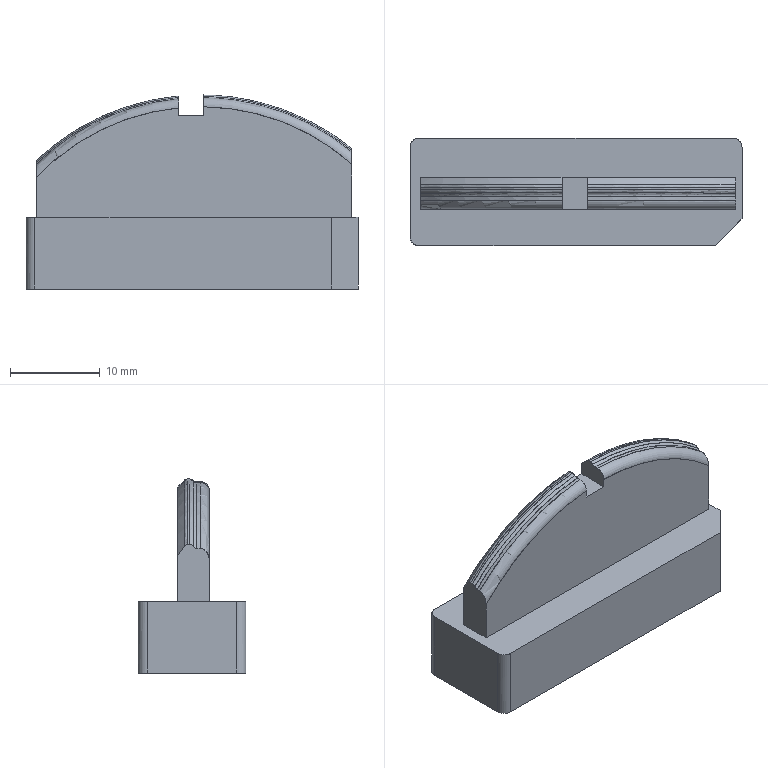NC program | PowerMill | posted with a generic post | part box 37 x 12 x 21.629 mm
Lines 9637 to 10369 of 105205:
N9734 M6
N9735 S18000 M03
N9736 G00 G90 X0.0 Y0.0
N9737 G43 Z10.799 H4
N9738
N9739 G05 P10000 R8
N9740 X18.17 Y-2.7087
N9741 Z-7.108
N9742 G01 Z-8.308 F1200.0
N9743 X18.1683 Y-2.7105 Z-8.3117 F2000.0
N9744 X18.1532 Y-2.7256 Z-8.3479
N9745 X18.1406 Y-2.7382 Z-8.3861
N9746 X18.0351 Y-2.8012 Z-8.5541
N9747 X18.0427 Y-2.7936 Z-8.51
N9748 X18.0532 Y-2.7832 Z-8.461
N9749 X18.0669 Y-2.7695 Z-8.407
N9750 X18.0841 Y-2.7522 Z-8.349
N9751 X18.1045 Y-2.7319 Z-8.2901
N9752 X18.1262 Y-2.7102 Z-8.2358
N9753 X18.1484 Y-2.6879 Z-8.1874
N9754 X18.1708 Y-2.6655 Z-8.1449
N9755 X18.1932 Y-2.6432 Z-8.1081
N9756 X18.2154 Y-2.621 Z-8.0766
N9757 X18.2375 Y-2.5989 Z-8.0501
N9758 X18.2475 Y-2.5889 Z-8.0395
N9759 X18.2796 Y-2.5143 Z-7.9042
N9760 X18.2615 Y-2.5324 Z-7.9174
N9761 X18.2384 Y-2.5556 Z-7.9379
N9762 X18.2136 Y-2.5803 Z-7.964
N9763 X18.1873 Y-2.6066 Z-7.9963
N9764 X18.1599 Y-2.634 Z-8.0349
N9765 X18.1352 Y-2.6587 Z-8.0744
N9766 X18.1154 Y-2.6786 Z-8.1103
N9767 X18.099 Y-2.6949 Z-8.1432
N9768 X18.0758 Y-2.7182 Z-8.1962
N9769 X18.0539 Y-2.7401 Z-8.2535
N9770 X18.0336 Y-2.7603 Z-8.3147
N9771 X18.0152 Y-2.7787 Z-8.3796
N9772 X17.9989 Y-2.795 Z-8.4477
N9773 X17.985 Y-2.8089 Z-8.5178
N9774 X17.9739 Y-2.8201 Z-8.5888
N9775 X17.9656 Y-2.8284 Z-8.6585
N9776 X17.9111 Y-2.8404 Z-8.6991
N9777 X17.9183 Y-2.8332 Z-8.6235
N9778 X17.9284 Y-2.8231 Z-8.5476
N9779 X17.9412 Y-2.8103 Z-8.4725
N9780 X17.9566 Y-2.7949 Z-8.3991
N9781 X17.9744 Y-2.7771 Z-8.3281
N9782 X17.9943 Y-2.7572 Z-8.26
N9783 X18.0159 Y-2.7357 Z-8.1964
N9784 X18.0379 Y-2.7136 Z-8.1395
N9785 X18.0616 Y-2.6899 Z-8.0864
N9786 X18.0865 Y-2.665 Z-8.0376
N9787 X18.1125 Y-2.639 Z-7.993
N9788 X18.1308 Y-2.6207 Z-7.9651
N9789 X18.1519 Y-2.5996 Z-7.9355
N9790 X18.1778 Y-2.5737 Z-7.9027
N9791 X18.206 Y-2.5455 Z-7.8715
N9792 X18.2333 Y-2.5182 Z-7.8455
N9793 X18.2593 Y-2.4922 Z-7.8249
N9794 X18.2841 Y-2.4674 Z-7.8092
N9795 X18.3077 Y-2.4438 Z-7.7982
N9796 X18.3097 Y-2.4418 Z-7.7974
N9797 X18.3331 Y-2.376 Z-7.7084
N9798 X18.3251 Y-2.3839 Z-7.711
N9799 X18.295 Y-2.4141 Z-7.7229
N9800 X18.2652 Y-2.4439 Z-7.7386
N9801 X18.2357 Y-2.4733 Z-7.7583
N9802 X18.2073 Y-2.5017 Z-7.7814
N9803 X18.1799 Y-2.5292 Z-7.8074
N9804 X18.153 Y-2.556 Z-7.8359
N9805 X18.1257 Y-2.5834 Z-7.8689
N9806 X18.0984 Y-2.6107 Z-7.9069
N9807 X18.0711 Y-2.638 Z-7.9504
N9808 X18.0437 Y-2.6654 Z-7.9997
N9809 X18.0166 Y-2.6925 Z-8.0547
N9810 X17.9915 Y-2.7176 Z-8.1125
N9811 X17.9681 Y-2.741 Z-8.1738
N9812 X17.9468 Y-2.7623 Z-8.238
N9813 X17.9289 Y-2.7801 Z-8.3002
N9814 X17.913 Y-2.7961 Z-8.3654
N9815 X17.8984 Y-2.8107 Z-8.436
N9816 X17.885 Y-2.8241 Z-8.5139
N9817 X17.8742 Y-2.8349 Z-8.5926
N9818 X17.8666 Y-2.8425 Z-8.6652
N9819 X17.8616 Y-2.8474 Z-8.7339
N9820 X17.815 Y-2.8516 Z-8.7667
N9821 X17.8195 Y-2.8471 Z-8.6835
N9822 X17.8268 Y-2.8398 Z-8.5992
N9823 X17.8367 Y-2.8299 Z-8.5167
N9824 X17.8489 Y-2.8177 Z-8.4374
N9825 X17.8632 Y-2.8034 Z-8.3621
N9826 X17.8794 Y-2.7872 Z-8.2913
N9827 X17.8973 Y-2.7694 Z-8.2252
N9828 X17.9172 Y-2.7494 Z-8.1617
N9829 X17.9398 Y-2.7268 Z-8.0995
N9830 X17.9644 Y-2.7022 Z-8.0403
N9831 X17.9908 Y-2.6759 Z-7.9844
N9832 X18.0188 Y-2.6478 Z-7.932
N9833 X18.0487 Y-2.618 Z-7.8826
N9834 X18.0797 Y-2.5869 Z-7.8367
N9835 X18.1104 Y-2.5563 Z-7.7965
N9836 X18.1407 Y-2.526 Z-7.7617
N9837 X18.1706 Y-2.4961 Z-7.732
N9838 X18.2012 Y-2.4655 Z-7.7062
N9839 X18.2333 Y-2.4334 Z-7.6827
N9840 X18.2636 Y-2.4031 Z-7.6645
N9841 X18.2922 Y-2.3745 Z-7.6511
N9842 X18.3194 Y-2.3473 Z-7.642
N9843 X18.3453 Y-2.3213 Z-7.6371
N9844 X18.3512 Y-2.3155 Z-7.6366
N9845 X18.3718 Y-2.2524 Z-7.5716
N9846 X18.3541 Y-2.2702 Z-7.5707
N9847 X18.342 Y-2.2822 Z-7.5722
N9848 X18.3109 Y-2.3133 Z-7.5787
N9849 X18.2793 Y-2.3449 Z-7.5894
N9850 X18.2472 Y-2.377 Z-7.6042
N9851 X18.2146 Y-2.4096 Z-7.6234
N9852 X18.1815 Y-2.4427 Z-7.6471
N9853 X18.148 Y-2.4762 Z-7.6755
N9854 X18.1141 Y-2.5101 Z-7.7088
N9855 X18.0801 Y-2.5441 Z-7.7468
N9856 X18.0464 Y-2.5779 Z-7.7895
N9857 X18.0137 Y-2.6105 Z-7.8358
N9858 X17.9862 Y-2.6381 Z-7.8794
N9859 X17.9577 Y-2.6665 Z-7.9301
N9860 X17.931 Y-2.6932 Z-7.9838
N9861 X17.9062 Y-2.7181 Z-8.0408
N9862 X17.8832 Y-2.7411 Z-8.1009
N9863 X17.8621 Y-2.7621 Z-8.1644
N9864 X17.843 Y-2.7812 Z-8.2312
N9865 X17.8259 Y-2.7983 Z-8.3014
N9866 X17.8109 Y-2.8133 Z-8.3752
N9867 X17.7981 Y-2.8261 Z-8.4525
N9868 X17.7875 Y-2.8367 Z-8.5334
N9869 X17.7793 Y-2.8449 Z-8.6179
N9870 X17.7736 Y-2.8506 Z-8.7058
N9871 X17.7704 Y-2.8538 Z-8.7969
N9872 X17.7273 Y-2.8545 Z-8.8067
N9873 X17.7293 Y-2.8525 Z-8.714
N9874 X17.7338 Y-2.848 Z-8.6242
N9875 X17.7408 Y-2.841 Z-8.5379
N9876 X17.7503 Y-2.8315 Z-8.4551
N9877 X17.762 Y-2.8198 Z-8.3759
N9878 X17.776 Y-2.8058 Z-8.3003
N9879 X17.7921 Y-2.7897 Z-8.2283
N9880 X17.8102 Y-2.7716 Z-8.1597
N9881 X17.8304 Y-2.7514 Z-8.0945
N9882 X17.8524 Y-2.7294 Z-8.0327
N9883 X17.8764 Y-2.7054 Z-7.9741
N9884 X17.9002 Y-2.6816 Z-7.9227
N9885 X17.9261 Y-2.6557 Z-7.8735
N9886 X17.955 Y-2.6268 Z-7.8252
N9887 X17.987 Y-2.5948 Z-7.7778
N9888 X18.0222 Y-2.5596 Z-7.7313
N9889 X18.0608 Y-2.521 Z-7.6857
N9890 X18.081 Y-2.5008 Z-7.6637
N9891 X18.0979 Y-2.4839 Z-7.647
N9892 X18.1152 Y-2.4666 Z-7.6313
N9893 X18.1388 Y-2.443 Z-7.6111
N9894 X18.1567 Y-2.4251 Z-7.5966
N9895 X18.1748 Y-2.407 Z-7.5828
N9896 X18.1933 Y-2.3885 Z-7.5701
N9897 X18.2124 Y-2.3694 Z-7.5589
N9898 X18.24 Y-2.3418 Z-7.5443
N9899 X18.2682 Y-2.3136 Z-7.5319
N9900 X18.297 Y-2.2848 Z-7.5226
N9901 X18.3262 Y-2.2556 Z-7.5168
N9902 X18.3557 Y-2.2261 Z-7.514
N9903 X18.3853 Y-2.1965 Z-7.5132
N9904 X18.3887 Y-2.1931
N9905 X18.4014 Y-2.138 Z-7.4637
N9906 X18.3823 Y-2.1571 Z-7.4599
N9907 X18.355 Y-2.1843 Z-7.4579
N9908 X18.326 Y-2.2134 Z-7.4597
N9909 X18.295 Y-2.2444 Z-7.4654
N9910 X18.2619 Y-2.2775 Z-7.4754
N9911 X18.2366 Y-2.3028 Z-7.4854
N9912 X18.2071 Y-2.3323 Z-7.5
N9913 X18.1781 Y-2.3612 Z-7.5167
N9914 X18.1462 Y-2.3932 Z-7.5375
N9915 X18.1183 Y-2.421 Z-7.5577
N9916 X18.0862 Y-2.4532 Z-7.5837
N9917 X18.0478 Y-2.4916 Z-7.6189
N9918 X18.0104 Y-2.529 Z-7.6579
N9919 X17.9749 Y-2.5644 Z-7.6998
N9920 X17.942 Y-2.5974 Z-7.7438
N9921 X17.9118 Y-2.6275 Z-7.7893
N9922 X17.8837 Y-2.6556 Z-7.8373
N9923 X17.8563 Y-2.683 Z-7.8901
N9924 X17.8307 Y-2.7087 Z-7.9462
N9925 X17.8069 Y-2.7325 Z-8.0055
N9926 X17.785 Y-2.7544 Z-8.0681
N9927 X17.765 Y-2.7744 Z-8.1341
N9928 X17.747 Y-2.7924 Z-8.2035
N9929 X17.7312 Y-2.8082 Z-8.2762
N9930 X17.7175 Y-2.8219 Z-8.3522
N9931 X17.7061 Y-2.8333 Z-8.4316
N9932 X17.697 Y-2.8423 Z-8.514
N9933 X17.691 Y-2.8484 Z-8.5919
N9934 X17.6866 Y-2.8527 Z-8.6814
N9935 X17.6848 Y-2.8545 Z-8.7759
N9936 Z-8.8163
N9937 X17.6424 Z-8.8258
N9938 Z-8.7397
N9939 X17.6441 Y-2.8529 Z-8.6473
N9940 X17.6483 Y-2.8486 Z-8.5582
N9941 X17.6551 Y-2.8418 Z-8.4723
N9942 X17.6644 Y-2.8326 Z-8.3897
N9943 X17.676 Y-2.821 Z-8.3104
N9944 X17.6899 Y-2.807 Z-8.2343
N9945 X17.706 Y-2.7909 Z-8.1614
N9946 X17.7243 Y-2.7726 Z-8.0916
N9947 X17.7424 Y-2.7545 Z-8.0318
N9948 X17.763 Y-2.734 Z-7.9729
N9949 X17.7865 Y-2.7105 Z-7.9145
N9950 X17.8127 Y-2.6842 Z-7.8573
N9951 X17.8411 Y-2.6558 Z-7.8027
N9952 X17.8712 Y-2.6257 Z-7.7514
N9953 X17.9027 Y-2.5943 Z-7.7039
N9954 X17.9351 Y-2.5619 Z-7.6604
N9955 X17.9681 Y-2.5288 Z-7.6214
N9956 X18.0024 Y-2.4945 Z-7.5857
N9957 X18.0407 Y-2.4562 Z-7.5508
N9958 X18.0812 Y-2.4158 Z-7.5185
N9959 X18.1239 Y-2.373 Z-7.489
N9960 X18.1689 Y-2.328 Z-7.4623
N9961 X18.2163 Y-2.2807 Z-7.4384
N9962 X18.2454 Y-2.2515 Z-7.4266
N9963 X18.2777 Y-2.2192 Z-7.417
N9964 X18.3117 Y-2.1852 Z-7.4104
N9965 X18.342 Y-2.1549 Z-7.4077
N9966 X18.3685 Y-2.1285 Z-7.4078
N9967 X18.3917 Y-2.1052 Z-7.4097
N9968 X18.4104 Y-2.0865 Z-7.4141
N9969 X18.4154 Y-2.0816 Z-7.4159
N9970 X18.4249 Y-2.0296 Z-7.3755
N9971 X18.4039 Y-2.0506 Z-7.3687
N9972 X18.3759 Y-2.0786 Z-7.3634
N9973 X18.3456 Y-2.1089 Z-7.3614
N9974 X18.3128 Y-2.1417 Z-7.363
N9975 X18.2774 Y-2.1771 Z-7.3685
N9976 X18.2392 Y-2.2153 Z-7.3782
N9977 X18.1983 Y-2.2563 Z-7.3925
N9978 X18.1552 Y-2.2993 Z-7.4115
N9979 X18.1128 Y-2.3417 Z-7.434
N9980 X18.075 Y-2.3795 Z-7.4572
N9981 X18.0411 Y-2.4135 Z-7.4808
N9982 X18.0013 Y-2.4532 Z-7.5123
N9983 X17.9633 Y-2.4912 Z-7.5468
N9984 X17.927 Y-2.5275 Z-7.5844
N9985 X17.8924 Y-2.5621 Z-7.6252
N9986 X17.8595 Y-2.595 Z-7.6691
N9987 X17.8284 Y-2.6261 Z-7.7161
N9988 X17.799 Y-2.6555 Z-7.7664
N9989 X17.7714 Y-2.6832 Z-7.8198
N9990 X17.7455 Y-2.7091 Z-7.8766
N9991 X17.7214 Y-2.7331 Z-7.9364
N9992 X17.6994 Y-2.7551 Z-7.9992
N9993 X17.6794 Y-2.7751 Z-8.0649
N9994 X17.6616 Y-2.793 Z-8.1336
N9995 X17.6458 Y-2.8087 Z-8.2054
N9996 X17.6323 Y-2.8222 Z-8.2806
N9997 X17.6211 Y-2.8334 Z-8.3592
N9998 X17.6121 Y-2.8424 Z-8.4414
N9999 X17.6055 Y-2.849 Z-8.5276
N10000 X17.6015 Y-2.8531 Z-8.6177
N10001 X17.5999 Y-2.8546 Z-8.7122
N10002 Z-8.8354
N10003 X17.5575 Z-8.827
N10004 Z-8.6741
N10005 X17.5591 Y-2.853 Z-8.5811
N10006 X17.5633 Y-2.8488 Z-8.4911
N10007 X17.5699 Y-2.8422 Z-8.4046
N10008 X17.579 Y-2.8331 Z-8.3217
N10009 X17.5904 Y-2.8217 Z-8.2424
N10010 X17.6041 Y-2.808 Z-8.1668
N10011 X17.6198 Y-2.7923 Z-8.0947
N10012 X17.6376 Y-2.7745 Z-8.0261
N10013 X17.6575 Y-2.7546 Z-7.9608
N10014 X17.6792 Y-2.7328 Z-7.8989
N10015 X17.7029 Y-2.7092 Z-7.8402
N10016 X17.7285 Y-2.6836 Z-7.7846
N10017 X17.7561 Y-2.656 Z-7.7318
N10018 X17.7859 Y-2.6262 Z-7.6811
N10019 X17.8175 Y-2.5946 Z-7.6335
N10020 X17.8508 Y-2.5613 Z-7.5891
N10021 X17.8858 Y-2.5263 Z-7.548
N10022 X17.9225 Y-2.4896 Z-7.51
N10023 X17.9609 Y-2.4512 Z-7.4752
N10024 X18.001 Y-2.4111 Z-7.4436
N10025 X18.0428 Y-2.3693 Z-7.4152
N10026 X18.0835 Y-2.3286 Z-7.3914
N10027 X18.1283 Y-2.2838 Z-7.3686
N10028 X18.1741 Y-2.238 Z-7.3491
N10029 X18.2177 Y-2.1944 Z-7.3344
N10030 X18.2586 Y-2.1535 Z-7.3242
N10031 X18.2966 Y-2.1155 Z-7.3182
N10032 X18.3319 Y-2.0802 Z-7.3162
N10033 X18.3646 Y-2.0475 Z-7.3179
N10034 X18.3949 Y-2.0172 Z-7.3229
N10035 X18.4228 Y-1.9893 Z-7.3312
N10036 X18.4342 Y-1.9779 Z-7.3358
N10037 X18.4422 Y-1.9275 Z-7.3004
N10038 X18.4393 Y-1.9304 Z-7.2991
N10039 X18.4086 Y-1.9611 Z-7.2878
N10040 X18.3764 Y-1.9933 Z-7.28
N10041 X18.3424 Y-2.0272 Z-7.2757
N10042 X18.3065 Y-2.0632 Z-7.2751
N10043 X18.2684 Y-2.1013 Z-7.2783
N10044 X18.2277 Y-2.142 Z-7.2855
N10045 X18.1841 Y-2.1856 Z-7.2972
N10046 X18.1313 Y-2.2384 Z-7.3149
N10047 X18.0837 Y-2.286 Z-7.3344
N10048 X18.04 Y-2.3296 Z-7.3561
N10049 X17.9992 Y-2.3705 Z-7.3803
N10050 X17.9575 Y-2.4122 Z-7.4091
N10051 X17.9167 Y-2.4529 Z-7.4416
N10052 X17.8779 Y-2.4918 Z-7.477
N10053 X17.841 Y-2.5287 Z-7.5154
N10054 X17.806 Y-2.5637 Z-7.5567
N10055 X17.7729 Y-2.5968 Z-7.6009
N10056 X17.7417 Y-2.628 Z-7.648
N10057 X17.7124 Y-2.6572 Z-7.6981
N10058 X17.6851 Y-2.6846 Z-7.7511
N10059 X17.6596 Y-2.7101 Z-7.8071
N10060 X17.6373 Y-2.7324 Z-7.8626
N10061 X17.6151 Y-2.7546 Z-7.9253
N10062 X17.5952 Y-2.7744 Z-7.9902
N10063 X17.5775 Y-2.7922 Z-8.058
N10064 X17.5619 Y-2.8078 Z-8.129
N10065 X17.5484 Y-2.8213 Z-8.2035
N10066 X17.5371 Y-2.8326 Z-8.2821
N10067 X17.5279 Y-2.8418 Z-8.3651
N10068 X17.521 Y-2.8486 Z-8.4512
N10069 X17.5168 Y-2.8529 Z-8.5386
N10070 X17.5151 Y-2.8546 Z-8.6298
N10071 Z-8.8061
N10072 X17.4727 Y-2.8545 Z-8.7853
N10073 Z-8.5897
N10074 X17.4745 Y-2.8527 Z-8.498
N10075 X17.4789 Y-2.8483 Z-8.409
N10076 X17.4859 Y-2.8414 Z-8.3235
N10077 X17.4952 Y-2.8321 Z-8.2419
N10078 X17.5067 Y-2.8205 Z-8.1643
N10079 X17.5206 Y-2.8066 Z-8.0892
N10080 X17.5367 Y-2.7905 Z-8.0173
N10081 X17.5549 Y-2.7724 Z-7.9487
N10082 X17.5751 Y-2.7522 Z-7.8834
N10083 X17.5973 Y-2.73 Z-7.8212
N10084 X17.6214 Y-2.7059 Z-7.7622
N10085 X17.6474 Y-2.6799 Z-7.7064
N10086 X17.6753 Y-2.652 Z-7.6537
N10087 X17.7049 Y-2.6223 Z-7.6041
N10088 X17.7364 Y-2.5908 Z-7.5575
N10089 X17.7696 Y-2.5576 Z-7.514
N10090 X17.8046 Y-2.5226 Z-7.4735
N10091 X17.8412 Y-2.486 Z-7.436
N10092 X17.8795 Y-2.4478 Z-7.4016
N10093 X17.9194 Y-2.4078 Z-7.3703
N10094 X17.9614 Y-2.3658 Z-7.3419
N10095 X18.0054 Y-2.3218 Z-7.3165
N10096 X18.0514 Y-2.2758 Z-7.2942
N10097 X18.0994 Y-2.2279 Z-7.2752
N10098 X18.1492 Y-2.178 Z-7.2595
N10099 X18.182 Y-2.1452 Z-7.2513
N10100 X18.2171 Y-2.1101 Z-7.244
N10101 X18.2576 Y-2.0697 Z-7.2377
N10102 X18.2972 Y-2.0301 Z-7.2347
N10103 X18.334 Y-1.9932 Z-7.2351
N10104 X18.368 Y-1.9593 Z-7.2391
N10105 X18.3993 Y-1.9279 Z-7.2462
N10106 X18.4282 Y-1.899 Z-7.2565
N10107 X18.4516 Y-1.8757 Z-7.2679
N10108 X18.4582 Y-1.8266 Z-7.2388
N10109 X18.4373 Y-1.8475 Z-7.2266
N10110 X18.411 Y-1.8739 Z-7.2151
N10111 X18.3816 Y-1.9032 Z-7.2063
N10112 X18.3486 Y-1.9362 Z-7.2002
N10113 X18.3105 Y-1.9743 Z-7.1969
N10114 X18.2843 Y-2.0005 Z-7.1966
N10115 X18.2549 Y-2.0299 Z-7.1983
N10116 X18.2186 Y-2.0662 Z-7.202
N10117 X18.1893 Y-2.0955 Z-7.206
N10118 X18.1601 Y-2.1247 Z-7.2111
N10119 X18.1095 Y-2.1753 Z-7.223
N10120 X18.06 Y-2.2248 Z-7.2385
N10121 X18.012 Y-2.2729 Z-7.2576
N10122 X17.9654 Y-2.3194 Z-7.2802
N10123 X17.9205 Y-2.3643 Z-7.3061
N10124 X17.8786 Y-2.4062 Z-7.3344
N10125 X17.8383 Y-2.4466 Z-7.3659
N10126 X17.7995 Y-2.4853 Z-7.4006
N10127 X17.7624 Y-2.5225 Z-7.4386
N10128 X17.7269 Y-2.5579 Z-7.4797
N10129 X17.6932 Y-2.5916 Z-7.5239
N10130 X17.6614 Y-2.6234 Z-7.5712
N10131 X17.6314 Y-2.6534 Z-7.6215
N10132 X17.6033 Y-2.6815 Z-7.6747
N10133 X17.5773 Y-2.7076 Z-7.7308
N10134 X17.5532 Y-2.7316 Z-7.7897
N10135 X17.5314 Y-2.7535 Z-7.8513
N10136 X17.5113 Y-2.7735 Z-7.9163
N10137 X17.4934 Y-2.7915 Z-7.9846
N10138 X17.4775 Y-2.8073 Z-8.0562
N10139 X17.4638 Y-2.821 Z-8.1312
N10140 X17.4523 Y-2.8325 Z-8.2097
N10141 X17.4431 Y-2.8417 Z-8.2919
N10142 X17.4363 Y-2.8485 Z-8.3779
N10143 X17.432 Y-2.8528 Z-8.4676
N10144 X17.4302 Y-2.8546 Z-8.5611
N10145 Z-8.7643
N10146 X17.3878 Z-8.7417
N10147 Z-8.5199
N10148 X17.3898 Y-2.8526 Z-8.4258
N10149 X17.3942 Y-2.8482 Z-8.3363
N10150 X17.4011 Y-2.8412 Z-8.251
N10151 X17.4104 Y-2.832 Z-8.1696
N10152 X17.422 Y-2.8204 Z-8.0918
N10153 X17.4358 Y-2.8066 Z-8.0174
N10154 X17.4519 Y-2.7905 Z-7.9461
N10155 X17.4696 Y-2.7728 Z-7.8793
N10156 X17.4896 Y-2.7528 Z-7.8148
N10157 X17.5116 Y-2.7308 Z-7.7531
N10158 X17.5356 Y-2.7068 Z-7.6942
N10159 X17.5616 Y-2.6808 Z-7.6383
N10160 X17.5895 Y-2.6528 Z-7.5854
N10161 X17.6194 Y-2.623 Z-7.5354
N10162 X17.6511 Y-2.5913 Z-7.4884
N10163 X17.6847 Y-2.5577 Z-7.4444
N10164 X17.72 Y-2.5224 Z-7.4035
N10165 X17.7572 Y-2.4852 Z-7.3657
N10166 X17.7961 Y-2.4463 Z-7.3309
N10167 X17.8367 Y-2.4057 Z-7.2993
N10168 X17.879 Y-2.3634 Z-7.2708
N10169 X17.923 Y-2.3194 Z-7.2455
N10170 X17.9686 Y-2.2738 Z-7.2234
N10171 X18.0155 Y-2.2269 Z-7.2045
N10172 X18.0661 Y-2.1763 Z-7.1882
N10173 X18.1176 Y-2.1248 Z-7.1757
N10174 X18.1699 Y-2.0725 Z-7.167
N10175 X18.2229 Y-2.0195 Z-7.1622
N10176 X18.2764 Y-1.966 Z-7.1614
N10177 X18.3103 Y-1.9321 Z-7.1629
N10178 X18.3496 Y-1.8928 Z-7.167
N10179 X18.3828 Y-1.8596 Z-7.1735
N10180 X18.4119 Y-1.8305 Z-7.1825
N10181 X18.4378 Y-1.8046 Z-7.1941
N10182 X18.4611 Y-1.7813 Z-7.2083
N10183 X18.4643 Y-1.7781 Z-7.2106
N10184 X18.4706 Y-1.7293 Z-7.1856
N10185 X18.4628 Y-1.7372 Z-7.18
N10186 X18.4371 Y-1.7629 Z-7.1644
N10187 X18.4088 Y-1.7912 Z-7.1514
N10188 X18.3775 Y-1.8225 Z-7.1411
N10189 X18.3426 Y-1.8574 Z-7.1334
N10190 X18.3028 Y-1.8971 Z-7.1285
N10191 X18.2449 Y-1.955 Z-7.1255
N10192 X18.1885 Y-2.0114 Z-7.1265
N10193 X18.1336 Y-2.0664 Z-7.1313
N10194 X18.0801 Y-2.1198 Z-7.1398
N10195 X18.0282 Y-2.1717 Z-7.152
N10196 X17.9778 Y-2.2222 Z-7.1677
N10197 X17.93 Y-2.2699 Z-7.1865
N10198 X17.8838 Y-2.3161 Z-7.2087
N10199 X17.8393 Y-2.3607 Z-7.2342
N10200 X17.7965 Y-2.4035 Z-7.2629
N10201 X17.7553 Y-2.4446 Z-7.2948
N10202 X17.716 Y-2.4839 Z-7.3299
N10203 X17.6785 Y-2.5214 Z-7.368
N10204 X17.6429 Y-2.557 Z-7.409
N10205 X17.6092 Y-2.5908 Z-7.4531
N10206 X17.5774 Y-2.6226 Z-7.4999
N10207 X17.5476 Y-2.6524 Z-7.5496
N10208 X17.5198 Y-2.6802 Z-7.602
N10209 X17.494 Y-2.706 Z-7.6572
N10210 X17.47 Y-2.7299 Z-7.7155
N10211 X17.448 Y-2.752 Z-7.777
N10212 X17.4278 Y-2.7721 Z-7.8418
N10213 X17.4097 Y-2.7903 Z-7.9101
N10214 X17.3936 Y-2.8063 Z-7.9817
N10215 X17.3797 Y-2.8202 Z-8.0569
N10216 X17.368 Y-2.8319 Z-8.1356
N10217 X17.3586 Y-2.8413 Z-8.2178
N10218 X17.3517 Y-2.8483 Z-8.3033
N10219 X17.3472 Y-2.8527 Z-8.3921
N10220 X17.3454 Y-2.8546 Z-8.4834
N10221 Z-8.7055
N10222 X17.303 Z-8.6694
N10223 Z-8.4469
N10224 X17.3044 Y-2.8532 Z-8.3672
N10225 X17.308 Y-2.8496 Z-8.2855
N10226 X17.3141 Y-2.8434 Z-8.2033
N10227 X17.3226 Y-2.8349 Z-8.1245
N10228 X17.3335 Y-2.824 Z-8.0464
N10229 X17.3456 Y-2.812 Z-7.9761
N10230 X17.3606 Y-2.7969 Z-7.9036
N10231 X17.3778 Y-2.7797 Z-7.8344
N10232 X17.3971 Y-2.7604 Z-7.7684
N10233 X17.4184 Y-2.7392 Z-7.7055
N10234 X17.4416 Y-2.7159 Z-7.6457
N10235 X17.4669 Y-2.6907 Z-7.5891
N10236 X17.494 Y-2.6635 Z-7.5354
N10237 X17.523 Y-2.6345 Z-7.4848
N10238 X17.5539 Y-2.6037 Z-7.4371
N10239 X17.5866 Y-2.571 Z-7.3924
N10240 X17.6211 Y-2.5365 Z-7.3505
N10241 X17.6573 Y-2.5002 Z-7.3116
N10242 X17.6955 Y-2.4621 Z-7.2754
N10243 X17.7355 Y-2.422 Z-7.2421
N10244 X17.777 Y-2.3805 Z-7.2122
N10245 X17.8203 Y-2.3372 Z-7.1854
N10246 X17.8654 Y-2.2921 Z-7.1618
N10247 X17.9124 Y-2.2452 Z-7.1414
N10248 X17.9612 Y-2.1963 Z-7.1243
N10249 X18.0121 Y-2.1454 Z-7.1106
N10250 X18.065 Y-2.0926 Z-7.1004
N10251 X18.1162 Y-2.0413 Z-7.094
N10252 X18.1546 Y-2.003 Z-7.0913
N10253 X18.2 Y-1.9575 Z-7.0903
N10254 X18.2528 Y-1.9048 Z-7.0921
N10255 X18.3013 Y-1.8563 Z-7.0972
N10256 X18.3433 Y-1.8142 Z-7.1047
N10257 X18.3799 Y-1.7777 Z-7.1143
N10258 X18.4118 Y-1.7458 Z-7.1256
N10259 X18.4396 Y-1.7179 Z-7.1386
N10260 X18.4638 Y-1.6938 Z-7.153
N10261 X18.478 Y-1.6795 Z-7.1634
N10262 X18.4845 Y-1.6306 Z-7.1421
N10263 X18.4605 Y-1.6546 Z-7.1252
N10264 X18.4323 Y-1.6828 Z-7.1084
N10265 X18.4024 Y-1.7127 Z-7.0941
N10266 X18.3697 Y-1.7454 Z-7.0822
N10267 X18.333 Y-1.7821 Z-7.0727
N10268 X18.2909 Y-1.8242 Z-7.0655
N10269 X18.2484 Y-1.8667 Z-7.0605
N10270 X18.2058 Y-1.9093 Z-7.0567
N10271 X18.1536 Y-1.9615 Z-7.0549
N10272 X18.0979 Y-2.0172 Z-7.0568
N10273 X18.0416 Y-2.0735 Z-7.0625
N10274 X17.9882 Y-2.1269 Z-7.0717
N10275 X17.9386 Y-2.1765 Z-7.0838
N10276 X17.893 Y-2.2221 Z-7.0983
N10277 X17.8451 Y-2.27 Z-7.1174
N10278 X17.7988 Y-2.3163 Z-7.1397
N10279 X17.7543 Y-2.3608 Z-7.1653
N10280 X17.7115 Y-2.4036 Z-7.1941
N10281 X17.6704 Y-2.4447 Z-7.226
N10282 X17.6311 Y-2.484 Z-7.261
N10283 X17.5937 Y-2.5214 Z-7.299
N10284 X17.5581 Y-2.557 Z-7.3401
N10285 X17.5244 Y-2.5908 Z-7.3842
N10286 X17.4925 Y-2.6226 Z-7.4312
N10287 X17.4627 Y-2.6525 Z-7.4811
N10288 X17.4347 Y-2.6804 Z-7.5339
N10289 X17.4088 Y-2.7063 Z-7.5895
N10290 X17.3848 Y-2.7303 Z-7.6478
N10291 X17.3624 Y-2.7527 Z-7.7102
N10292 X17.3422 Y-2.7729 Z-7.7752
N10293 X17.3241 Y-2.791 Z-7.8432
N10294 X17.3082 Y-2.807 Z-7.9144
N10295 X17.2944 Y-2.8207 Z-7.9888
N10296 X17.2829 Y-2.8323 Z-8.0666
N10297 X17.2736 Y-2.8415 Z-8.148
N10298 X17.2668 Y-2.8483 Z-8.2333
N10299 X17.2624 Y-2.8527 Z-8.3226
N10300 X17.2605 Y-2.8546 Z-8.4163
N10301 Z-8.6332
N10302 X17.2182 Y-2.8545 Z-8.5971
N10303 Z-8.3742
N10304 X17.2201 Y-2.8526 Z-8.283
N10305 X17.2246 Y-2.8481 Z-8.1946
N10306 X17.2316 Y-2.841 Z-8.1095
N10307 X17.2411 Y-2.8316 Z-8.0278
N10308 X17.2529 Y-2.8198 Z-7.9496
N10309 X17.2669 Y-2.8058 Z-7.8749
N10310 X17.283 Y-2.7897 Z-7.8036
N10311 X17.3012 Y-2.7715 Z-7.7357
N10312 X17.3214 Y-2.7512 Z-7.671
N10313 X17.3436 Y-2.729 Z-7.6097
N10314 X17.3677 Y-2.7049 Z-7.5515
N10315 X17.3934 Y-2.6792 Z-7.4969
N10316 X17.4211 Y-2.6516 Z-7.445
N10317 X17.4508 Y-2.6219 Z-7.3957
N10318 X17.4824 Y-2.5903 Z-7.3492
N10319 X17.5159 Y-2.5568 Z-7.3054
N10320 X17.5514 Y-2.5213 Z-7.2645
N10321 X17.5888 Y-2.4839 Z-7.2266
N10322 X17.628 Y-2.4446 Z-7.1915
N10323 X17.6692 Y-2.4035 Z-7.1596
N10324 X17.7122 Y-2.3605 Z-7.1307
N10325 X17.7569 Y-2.3157 Z-7.105
N10326 X17.8035 Y-2.2692 Z-7.0826
N10327 X17.8518 Y-2.2209 Z-7.0635
N10328 X17.9018 Y-2.1709 Z-7.0478
N10329 X17.9534 Y-2.1193 Z-7.0356
N10330 X18.0065 Y-2.0662 Z-7.027
N10331 X18.0629 Y-2.0097 Z-7.0217
N10332 X18.121 Y-1.9517 Z-7.0202
N10333 X18.1807 Y-1.892 Z-7.0227
N10334 X18.242 Y-1.8307 Z-7.0291
N10335 X18.3052 Y-1.7675 Z-7.0397
N10336 X18.3468 Y-1.7259 Z-7.0496
N10337 X18.3845 Y-1.6882 Z-7.0621
N10338 X18.4189 Y-1.6538 Z-7.0772
N10339 X18.4504 Y-1.6223 Z-7.0948
N10340 X18.4794 Y-1.5933 Z-7.1149
N10341 X18.4894 Y-1.5833 Z-7.123
N10342 X18.4949 Y-1.5353 Z-7.1045
N10343 X18.4805 Y-1.5497 Z-7.0923
N10344 X18.4578 Y-1.5725 Z-7.0761
N10345 X18.4317 Y-1.5985 Z-7.0608
N10346 X18.4021 Y-1.6281 Z-7.0463
N10347 X18.3687 Y-1.6615 Z-7.0329
N10348 X18.3313 Y-1.699 Z-7.0206
N10349 X18.2895 Y-1.7408 Z-7.0096
N10350 X18.243 Y-1.7873 Z-7.0002
N10351 X18.1913 Y-1.8389 Z-6.9928
N10352 X18.1343 Y-1.896 Z-6.9879
N10353 X18.0723 Y-1.958 Z-6.9861
N10354 X18.016 Y-2.0143 Z-6.9877
N10355 X17.9611 Y-2.0692 Z-6.9928
N10356 X17.9077 Y-2.1226 Z-7.0017
N10357 X17.8559 Y-2.1743 Z-7.0142
N10358 X17.8059 Y-2.2243 Z-7.0301
N10359 X17.7578 Y-2.2725 Z-7.0495
N10360 X17.7114 Y-2.3188 Z-7.0722
N10361 X17.667 Y-2.3633 Z-7.098
N10362 X17.6244 Y-2.4059 Z-7.1269
N10363 X17.5837 Y-2.4465 Z-7.1589
N10364 X17.5449 Y-2.4853 Z-7.1938
N10365 X17.5079 Y-2.5223 Z-7.2317
N10366 X17.4728 Y-2.5575 Z-7.2725
N10367 X17.4394 Y-2.5909 Z-7.3162
N10368 X17.4077 Y-2.6225 Z-7.3628
N10369 X17.3779 Y-2.6523 Z-7.4125
N10370 X17.3499 Y-2.6803 Z-7.4651
N10371 X17.3239 Y-2.7064 Z-7.5208
N10372 X17.2997 Y-2.7306 Z-7.5796
N10373 X17.2775 Y-2.7528 Z-7.6415
N10374 X17.2573 Y-2.773 Z-7.7065
N10375 X17.2392 Y-2.7911 Z-7.7747
N10376 X17.2232 Y-2.8071 Z-7.8461
N10377 X17.2093 Y-2.8209 Z-7.9208
N10378 X17.1978 Y-2.8325 Z-7.9987
N10379 X17.1885 Y-2.8417 Z-8.0799
N10380 X17.1817 Y-2.8485 Z-8.1645
N10381 X17.1774 Y-2.8529 Z-8.2523
N10382 X17.1757 Y-2.8545 Z-8.3433
N10383 Y-2.8546 Z-8.5614
N10384 X17.1333 Y-2.8545 Z-8.526
N10385 Z-8.3071
N10386 X17.1351 Y-2.8527 Z-8.2157
N10387 X17.1395 Y-2.8483 Z-8.1275
N10388 X17.1465 Y-2.8414 Z-8.0426
N10389 X17.1558 Y-2.832 Z-7.9612
N10390 X17.1675 Y-2.8203 Z-7.8832
N10391 X17.1814 Y-2.8064 Z-7.8085
N10392 X17.1976 Y-2.7903 Z-7.7373
N10393 X17.2158 Y-2.7721 Z-7.6693
N10394 X17.236 Y-2.7518 Z-7.6046
N10395 X17.2582 Y-2.7296 Z-7.543
N10396 X17.2824 Y-2.7054 Z-7.4846
N10397 X17.3085 Y-2.6793 Z-7.4293
N10398 X17.3364 Y-2.6514 Z-7.3769
N10399 X17.3662 Y-2.6216 Z-7.3276
N10400 X17.3981 Y-2.5897 Z-7.2807
N10401 X17.4317 Y-2.5561 Z-7.237
N10402 X17.4671 Y-2.5207 Z-7.1962
N10403 X17.5043 Y-2.4835 Z-7.1582
N10404 X17.5434 Y-2.4444 Z-7.1233
N10405 X17.5844 Y-2.4034 Z-7.0913
N10406 X17.6272 Y-2.3606 Z-7.0624
N10407 X17.6719 Y-2.3159 Z-7.0366
N10408 X17.7185 Y-2.2694 Z-7.0141
N10409 X17.7669 Y-2.2209 Z-6.9948
N10410 X17.8172 Y-2.1706 Z-6.9789
N10411 X17.8693 Y-2.1185 Z-6.9664
N10412 X17.9233 Y-2.0645 Z-6.9575
N10413 X17.9791 Y-2.0087 Z-6.9522
N10414 X18.0272 Y-1.9606 Z-6.9507
N10415 X18.066 Y-1.9218 Z-6.9514
N10416 X18.1112 Y-1.8766 Z-6.9543
N10417 X18.1646 Y-1.8233 Z-6.9603
N10418 X18.2266 Y-1.7612 Z-6.9707
N10419 X18.2809 Y-1.7069 Z-6.983
N10420 X18.3269 Y-1.6609 Z-6.9961
N10421 X18.3663 Y-1.6215 Z-7.0099
N10422 X18.4003 Y-1.5876 Z-7.0241
N10423 X18.4296 Y-1.5582 Z-7.0387
N10424 X18.4549 Y-1.533 Z-7.0537
N10425 X18.4763 Y-1.5115 Z-7.069
N10426 X18.495 Y-1.4929 Z-7.0853
N10427 X18.4994 Y-1.4885 Z-7.0898
N10428 X18.5029 Y-1.4425 Z-7.0753
N10429 X18.484 Y-1.4614 Z-7.0573
N10430 X18.4591 Y-1.4863 Z-7.0379
N10431 X18.4306 Y-1.5148 Z-7.0199
N10432 X18.3974 Y-1.548 Z-7.0031
N10433 X18.3573 Y-1.5881 Z-6.9865
N10434 X18.2941 Y-1.6513 Z-6.9645
N10435 X18.2311 Y-1.7143 Z-6.9466
N10436 X18.1687 Y-1.7767 Z-6.9328
N10437 X18.1072 Y-1.8382 Z-6.9231
N10438 X18.0467 Y-1.8987 Z-6.9175
N10439 X17.9876 Y-1.9578 Z-6.9159
N10440 X17.9299 Y-2.0156 Z-6.9182
N10441 X17.8736 Y-2.0718 Z-6.9242
N10442 X17.821 Y-2.1244 Z-6.9336
N10443 X17.7696 Y-2.1758 Z-6.9464
N10444 X17.7199 Y-2.2255 Z-6.9626
N10445 X17.6718 Y-2.2736 Z-6.9822
N10446 X17.6255 Y-2.3199 Z-7.005
N10447 X17.5809 Y-2.3645 Z-7.031
N10448 X17.5381 Y-2.4073 Z-7.0603
N10449 X17.4971 Y-2.4483 Z-7.0926
N10450 X17.4579 Y-2.4875 Z-7.128
N10451 X17.4206 Y-2.5248 Z-7.1664
N10452 X17.3852 Y-2.5602 Z-7.2078
N10453 X17.3517 Y-2.5937 Z-7.2521
N10454 X17.3201 Y-2.6253 Z-7.2993
N10455 X17.2905 Y-2.6549 Z-7.3493
N10456 X17.2629 Y-2.6825 Z-7.402
N10457 X17.2372 Y-2.7082 Z-7.4575
N10458 X17.2135 Y-2.7319 Z-7.5156
N10459 X17.1919 Y-2.7535 Z-7.5763
N10460 X17.1714 Y-2.774 Z-7.6422
N10461 X17.1534 Y-2.792 Z-7.7102
N10462 X17.1375 Y-2.8079 Z-7.781
N10463 X17.1239 Y-2.8215 Z-7.8547
N10464 X17.1126 Y-2.8328 Z-7.9317
N10465 X17.1035 Y-2.8419 Z-8.0123
N10466 X17.0969 Y-2.8485 Z-8.0969